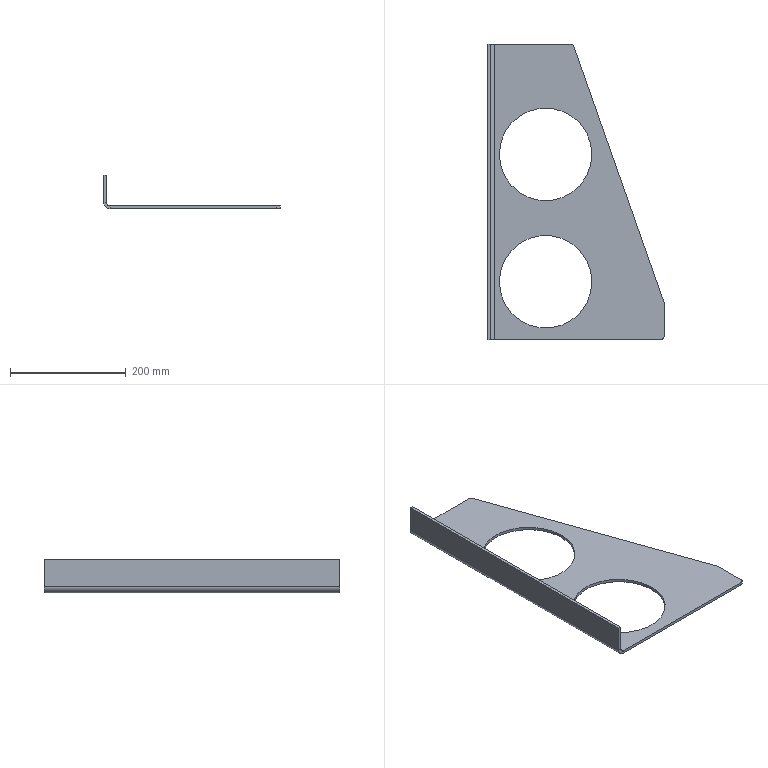Part | SolidWorks | features EdgeFlange 1, FlatPattern 1, ICE 1, SMBaseFlange 1, SheetMetal 1, UnFold 1 | 1 solid | 22 faces | box 305 x 510 x 58 mm | volume 526681 mm3 | plane 13 | cylinder 9 | commonest cylinder face diameters 160 x4 14 x3 12 x1 22 x1
STEP:
#1=CARTESIAN_POINT('',(415.,110.,-5.));
#2=VERTEX_POINT('',#1);
#3=CARTESIAN_POINT('',(255.,110.,-5.));
#4=VERTEX_POINT('',#3);
#5=CARTESIAN_POINT('',(335.,110.,-5.));
#6=DIRECTION('',(0.,0.,-1.));
#7=DIRECTION('',(-1.,0.,0.));
#8=AXIS2_PLACEMENT_3D('',#5,#6,#7);
#9=CIRCLE('',#8,80.);
#10=EDGE_CURVE('',#2,#4,#9,.T.);
#11=ORIENTED_EDGE('',*,*,#10,.T.);
#12=CARTESIAN_POINT('',(255.,110.,0.));
#13=VERTEX_POINT('',#12);
#14=CARTESIAN_POINT('',(255.,110.,-10.));
#15=DIRECTION('',(0.,0.,1.));
#16=VECTOR('',#15,1000.);
#17=LINE('',#14,#16);
#18=EDGE_CURVE('',#4,#13,#17,.T.);
#19=ORIENTED_EDGE('',*,*,#18,.T.);
#20=CARTESIAN_POINT('',(415.,110.,0.));
#21=VERTEX_POINT('',#20);
#22=CARTESIAN_POINT('',(335.,110.,0.));
#23=DIRECTION('',(0.,0.,1.));
#24=DIRECTION('',(1.,0.,0.));
#25=AXIS2_PLACEMENT_3D('',#22,#23,#24);
#26=CIRCLE('',#25,80.);
#27=EDGE_CURVE('',#13,#21,#26,.T.);
#28=ORIENTED_EDGE('',*,*,#27,.T.);
#29=CARTESIAN_POINT('',(415.,110.,-10.));
#30=DIRECTION('',(0.,0.,1.));
#31=VECTOR('',#30,1000.);
#32=LINE('',#29,#31);
#33=EDGE_CURVE('',#2,#21,#32,.T.);
#34=ORIENTED_EDGE('',*,*,#33,.F.);
#35=EDGE_LOOP('',(#11,#19,#28,#34));
#36=FACE_OUTER_BOUND('',#35,.T.);
#37=CARTESIAN_POINT('',(335.,110.,-10.));
#38=DIRECTION('',(0.,0.,1.));
#39=DIRECTION('',(1.,0.,0.));
#40=AXIS2_PLACEMENT_3D('',#37,#38,#39);
#41=CYLINDRICAL_SURFACE('',#40,80.);
#42=ADVANCED_FACE('',(#36),#41,.F.);
#43=CARTESIAN_POINT('',(415.,330.,-5.));
#44=VERTEX_POINT('',#43);
#45=CARTESIAN_POINT('',(255.,330.,-5.));
#46=VERTEX_POINT('',#45);
#47=CARTESIAN_POINT('',(335.,330.,-5.));
#48=DIRECTION('',(0.,0.,-1.));
#49=DIRECTION('',(-1.,0.,0.));
#50=AXIS2_PLACEMENT_3D('',#47,#48,#49);
#51=CIRCLE('',#50,80.);
#52=EDGE_CURVE('',#44,#46,#51,.T.);
#53=ORIENTED_EDGE('',*,*,#52,.T.);
#54=CARTESIAN_POINT('',(255.,330.,0.));
#55=VERTEX_POINT('',#54);
#56=CARTESIAN_POINT('',(255.,330.,-10.));
#57=DIRECTION('',(0.,0.,1.));
#58=VECTOR('',#57,1000.);
#59=LINE('',#56,#58);
#60=EDGE_CURVE('',#46,#55,#59,.T.);
#61=ORIENTED_EDGE('',*,*,#60,.T.);
#62=CARTESIAN_POINT('',(415.,330.,0.));
#63=VERTEX_POINT('',#62);
#64=CARTESIAN_POINT('',(335.,330.,0.));
#65=DIRECTION('',(0.,0.,1.));
#66=DIRECTION('',(1.,0.,0.));
#67=AXIS2_PLACEMENT_3D('',#64,#65,#66);
#68=CIRCLE('',#67,80.);
#69=EDGE_CURVE('',#55,#63,#68,.T.);
#70=ORIENTED_EDGE('',*,*,#69,.T.);
#71=CARTESIAN_POINT('',(415.,330.,-10.));
#72=DIRECTION('',(0.,0.,1.));
#73=VECTOR('',#72,1000.);
#74=LINE('',#71,#73);
#75=EDGE_CURVE('',#44,#63,#74,.T.);
#76=ORIENTED_EDGE('',*,*,#75,.F.);
#77=EDGE_LOOP('',(#53,#61,#70,#76));
#78=FACE_OUTER_BOUND('',#77,.T.);
#79=CARTESIAN_POINT('',(335.,330.,-10.));
#80=DIRECTION('',(0.,0.,1.));
#81=DIRECTION('',(1.,0.,0.));
#82=AXIS2_PLACEMENT_3D('',#79,#80,#81);
#83=CYLINDRICAL_SURFACE('',#82,80.);
#84=ADVANCED_FACE('',(#78),#83,.F.);
#85=CARTESIAN_POINT('',(246.,10.,0.));
#86=VERTEX_POINT('',#85);
#87=CARTESIAN_POINT('',(533.,10.,0.));
#88=VERTEX_POINT('',#87);
#89=CARTESIAN_POINT('',(235.,10.,0.));
#90=DIRECTION('',(1.,0.,0.));
#91=VECTOR('',#90,1000.);
#92=LINE('',#89,#91);
#93=EDGE_CURVE('',#86,#88,#92,.T.);
#94=ORIENTED_EDGE('',*,*,#93,.F.);
#95=CARTESIAN_POINT('',(246.,10.,-5.));
#96=VERTEX_POINT('',#95);
#97=CARTESIAN_POINT('',(246.,10.,0.));
#98=DIRECTION('',(0.,0.,-1.));
#99=VECTOR('',#98,1000.);
#100=LINE('',#97,#99);
#101=EDGE_CURVE('',#86,#96,#100,.T.);
#102=ORIENTED_EDGE('',*,*,#101,.T.);
#103=CARTESIAN_POINT('',(533.,10.,-5.));
#104=VERTEX_POINT('',#103);
#105=CARTESIAN_POINT('',(235.,10.,-5.));
#106=DIRECTION('',(1.,0.,0.));
#107=VECTOR('',#106,1000.);
#108=LINE('',#105,#107);
#109=EDGE_CURVE('',#96,#104,#108,.T.);
#110=ORIENTED_EDGE('',*,*,#109,.T.);
#111=CARTESIAN_POINT('',(533.,10.,-5.));
#112=DIRECTION('',(0.,0.,1.));
#113=VECTOR('',#112,1000.);
#114=LINE('',#111,#113);
#115=EDGE_CURVE('',#104,#88,#114,.T.);
#116=ORIENTED_EDGE('',*,*,#115,.T.);
#117=EDGE_LOOP('',(#94,#102,#110,#116));
#118=FACE_OUTER_BOUND('',#117,.T.);
#119=CARTESIAN_POINT('',(235.,10.,-5.));
#120=DIRECTION('',(0.,-1.,0.));
#121=DIRECTION('',(0.,0.,-1.));
#122=AXIS2_PLACEMENT_3D('',#119,#120,#121);
#123=PLANE('',#122);
#124=ADVANCED_FACE('',(#118),#123,.T.);
#125=ORIENTED_EDGE('',*,*,#10,.F.);
#126=CARTESIAN_POINT('',(335.,110.,-5.));
#127=DIRECTION('',(0.,0.,-1.));
#128=DIRECTION('',(-1.,0.,0.));
#129=AXIS2_PLACEMENT_3D('',#126,#127,#128);
#130=CIRCLE('',#129,80.);
#131=EDGE_CURVE('',#4,#2,#130,.T.);
#132=ORIENTED_EDGE('',*,*,#131,.F.);
#133=EDGE_LOOP('',(#125,#132));
#134=FACE_BOUND('',#133,.T.);
#135=ORIENTED_EDGE('',*,*,#52,.F.);
#136=CARTESIAN_POINT('',(335.,330.,-5.));
#137=DIRECTION('',(0.,0.,-1.));
#138=DIRECTION('',(-1.,0.,0.));
#139=AXIS2_PLACEMENT_3D('',#136,#137,#138);
#140=CIRCLE('',#139,80.);
#141=EDGE_CURVE('',#46,#44,#140,.T.);
#142=ORIENTED_EDGE('',*,*,#141,.F.);
#143=EDGE_LOOP('',(#135,#142));
#144=FACE_BOUND('',#143,.T.);
#145=ORIENTED_EDGE('',*,*,#109,.F.);
#146=CARTESIAN_POINT('',(246.,520.,-5.));
#147=VERTEX_POINT('',#146);
#148=CARTESIAN_POINT('',(246.,10.,-5.));
#149=DIRECTION('',(0.,1.,0.));
#150=VECTOR('',#149,1000.);
#151=LINE('',#148,#150);
#152=EDGE_CURVE('',#96,#147,#151,.T.);
#153=ORIENTED_EDGE('',*,*,#152,.T.);
#154=CARTESIAN_POINT('',(377.818,520.,-5.));
#155=VERTEX_POINT('',#154);
#156=CARTESIAN_POINT('',(235.,520.,-5.));
#157=DIRECTION('',(-1.,0.,0.));
#158=VECTOR('',#157,1000.);
#159=LINE('',#156,#158);
#160=EDGE_CURVE('',#155,#147,#159,.T.);
#161=ORIENTED_EDGE('',*,*,#160,.F.);
#162=CARTESIAN_POINT('',(384.422,515.322,-5.));
#163=VERTEX_POINT('',#162);
#164=CARTESIAN_POINT('',(377.818,513.,-5.));
#165=DIRECTION('',(0.,0.,1.));
#166=DIRECTION('',(1.,0.,0.));
#167=AXIS2_PLACEMENT_3D('',#164,#165,#166);
#168=CIRCLE('',#167,7.);
#169=EDGE_CURVE('',#163,#155,#168,.T.);
#170=ORIENTED_EDGE('',*,*,#169,.F.);
#171=CARTESIAN_POINT('',(539.604,73.92,-5.));
#172=VERTEX_POINT('',#171);
#173=CARTESIAN_POINT('',(384.422,515.322,-5.));
#174=DIRECTION('',(-0.3317,0.9434,0.));
#175=VECTOR('',#174,1000.);
#176=LINE('',#173,#175);
#177=EDGE_CURVE('',#172,#163,#176,.T.);
#178=ORIENTED_EDGE('',*,*,#177,.F.);
#179=CARTESIAN_POINT('',(540.,71.599,-5.));
#180=VERTEX_POINT('',#179);
#181=CARTESIAN_POINT('',(533.,71.599,-5.));
#182=DIRECTION('',(0.,0.,1.));
#183=DIRECTION('',(1.,0.,0.));
#184=AXIS2_PLACEMENT_3D('',#181,#182,#183);
#185=CIRCLE('',#184,7.);
#186=EDGE_CURVE('',#180,#172,#185,.T.);
#187=ORIENTED_EDGE('',*,*,#186,.F.);
#188=CARTESIAN_POINT('',(540.,17.,-5.));
#189=VERTEX_POINT('',#188);
#190=CARTESIAN_POINT('',(540.,17.,-5.));
#191=DIRECTION('',(0.,1.,0.));
#192=VECTOR('',#191,1000.);
#193=LINE('',#190,#192);
#194=EDGE_CURVE('',#189,#180,#193,.T.);
#195=ORIENTED_EDGE('',*,*,#194,.F.);
#196=CARTESIAN_POINT('',(533.,17.,-5.));
#197=DIRECTION('',(0.,0.,1.));
#198=DIRECTION('',(-1.,0.,0.));
#199=AXIS2_PLACEMENT_3D('',#196,#197,#198);
#200=CIRCLE('',#199,7.);
#201=EDGE_CURVE('',#104,#189,#200,.T.);
#202=ORIENTED_EDGE('',*,*,#201,.F.);
#203=EDGE_LOOP('',(#145,#153,#161,#170,#178,#187,#195,#202));
#204=FACE_OUTER_BOUND('',#203,.T.);
#205=CARTESIAN_POINT('',(533.,17.,-5.));
#206=DIRECTION('',(0.,0.,-1.));
#207=DIRECTION('',(-1.,0.,0.));
#208=AXIS2_PLACEMENT_3D('',#205,#206,#207);
#209=PLANE('',#208);
#210=ADVANCED_FACE('',(#134,#144,#204),#209,.T.);
#211=CARTESIAN_POINT('',(335.,330.,0.));
#212=DIRECTION('',(0.,0.,1.));
#213=DIRECTION('',(1.,0.,0.));
#214=AXIS2_PLACEMENT_3D('',#211,#212,#213);
#215=CIRCLE('',#214,80.);
#216=EDGE_CURVE('',#63,#55,#215,.T.);
#217=ORIENTED_EDGE('',*,*,#216,.F.);
#218=ORIENTED_EDGE('',*,*,#69,.F.);
#219=EDGE_LOOP('',(#217,#218));
#220=FACE_BOUND('',#219,.T.);
#221=CARTESIAN_POINT('',(335.,110.,0.));
#222=DIRECTION('',(0.,0.,1.));
#223=DIRECTION('',(1.,0.,0.));
#224=AXIS2_PLACEMENT_3D('',#221,#222,#223);
#225=CIRCLE('',#224,80.);
#226=EDGE_CURVE('',#21,#13,#225,.T.);
#227=ORIENTED_EDGE('',*,*,#226,.F.);
#228=ORIENTED_EDGE('',*,*,#27,.F.);
#229=EDGE_LOOP('',(#227,#228));
#230=FACE_BOUND('',#229,.T.);
#231=CARTESIAN_POINT('',(246.,520.,0.));
#232=VERTEX_POINT('',#231);
#233=CARTESIAN_POINT('',(246.,10.,0.));
#234=DIRECTION('',(0.,1.,0.));
#235=VECTOR('',#234,1000.);
#236=LINE('',#233,#235);
#237=EDGE_CURVE('',#86,#232,#236,.T.);
#238=ORIENTED_EDGE('',*,*,#237,.F.);
#239=ORIENTED_EDGE('',*,*,#93,.T.);
#240=CARTESIAN_POINT('',(540.,17.,0.));
#241=VERTEX_POINT('',#240);
#242=CARTESIAN_POINT('',(533.,17.,0.));
#243=DIRECTION('',(0.,0.,1.));
#244=DIRECTION('',(-1.,0.,0.));
#245=AXIS2_PLACEMENT_3D('',#242,#243,#244);
#246=CIRCLE('',#245,7.);
#247=EDGE_CURVE('',#88,#241,#246,.T.);
#248=ORIENTED_EDGE('',*,*,#247,.T.);
#249=CARTESIAN_POINT('',(540.,71.599,0.));
#250=VERTEX_POINT('',#249);
#251=CARTESIAN_POINT('',(540.,17.,0.));
#252=DIRECTION('',(0.,1.,0.));
#253=VECTOR('',#252,1000.);
#254=LINE('',#251,#253);
#255=EDGE_CURVE('',#241,#250,#254,.T.);
#256=ORIENTED_EDGE('',*,*,#255,.T.);
#257=CARTESIAN_POINT('',(539.604,73.92,0.));
#258=VERTEX_POINT('',#257);
#259=CARTESIAN_POINT('',(533.,71.599,0.));
#260=DIRECTION('',(0.,0.,1.));
#261=DIRECTION('',(1.,0.,0.));
#262=AXIS2_PLACEMENT_3D('',#259,#260,#261);
#263=CIRCLE('',#262,7.);
#264=EDGE_CURVE('',#250,#258,#263,.T.);
#265=ORIENTED_EDGE('',*,*,#264,.T.);
#266=CARTESIAN_POINT('',(384.422,515.322,0.));
#267=VERTEX_POINT('',#266);
#268=CARTESIAN_POINT('',(384.422,515.322,0.));
#269=DIRECTION('',(-0.3317,0.9434,0.));
#270=VECTOR('',#269,1000.);
#271=LINE('',#268,#270);
#272=EDGE_CURVE('',#258,#267,#271,.T.);
#273=ORIENTED_EDGE('',*,*,#272,.T.);
#274=CARTESIAN_POINT('',(377.818,520.,0.));
#275=VERTEX_POINT('',#274);
#276=CARTESIAN_POINT('',(377.818,513.,0.));
#277=DIRECTION('',(0.,0.,1.));
#278=DIRECTION('',(1.,0.,0.));
#279=AXIS2_PLACEMENT_3D('',#276,#277,#278);
#280=CIRCLE('',#279,7.);
#281=EDGE_CURVE('',#267,#275,#280,.T.);
#282=ORIENTED_EDGE('',*,*,#281,.T.);
#283=CARTESIAN_POINT('',(235.,520.,0.));
#284=DIRECTION('',(-1.,0.,0.));
#285=VECTOR('',#284,1000.);
#286=LINE('',#283,#285);
#287=EDGE_CURVE('',#275,#232,#286,.T.);
#288=ORIENTED_EDGE('',*,*,#287,.T.);
#289=EDGE_LOOP('',(#238,#239,#248,#256,#265,#273,#282,#288));
#290=FACE_OUTER_BOUND('',#289,.T.);
#291=CARTESIAN_POINT('',(533.,17.,0.));
#292=DIRECTION('',(0.,0.,-1.));
#293=DIRECTION('',(-1.,0.,0.));
#294=AXIS2_PLACEMENT_3D('',#291,#292,#293);
#295=PLANE('',#294);
#296=ADVANCED_FACE('',(#220,#230,#290),#295,.F.);
#297=CARTESIAN_POINT('',(246.,520.,0.));
#298=DIRECTION('',(0.,0.,-1.));
#299=VECTOR('',#298,1000.);
#300=LINE('',#297,#299);
#301=EDGE_CURVE('',#232,#147,#300,.T.);
#302=ORIENTED_EDGE('',*,*,#301,.F.);
#303=ORIENTED_EDGE('',*,*,#287,.F.);
#304=CARTESIAN_POINT('',(377.818,520.,-5.));
#305=DIRECTION('',(0.,0.,1.));
#306=VECTOR('',#305,1000.);
#307=LINE('',#304,#306);
#308=EDGE_CURVE('',#155,#275,#307,.T.);
#309=ORIENTED_EDGE('',*,*,#308,.F.);
#310=ORIENTED_EDGE('',*,*,#160,.T.);
#311=EDGE_LOOP('',(#302,#303,#309,#310));
#312=FACE_OUTER_BOUND('',#311,.T.);
#313=CARTESIAN_POINT('',(235.,520.,-5.));
#314=DIRECTION('',(0.,1.,0.));
#315=DIRECTION('',(-1.,0.,0.));
#316=AXIS2_PLACEMENT_3D('',#313,#314,#315);
#317=PLANE('',#316);
#318=ADVANCED_FACE('',(#312),#317,.T.);
#319=ORIENTED_EDGE('',*,*,#281,.F.);
#320=CARTESIAN_POINT('',(384.422,515.322,-5.));
#321=DIRECTION('',(0.,0.,1.));
#322=VECTOR('',#321,1000.);
#323=LINE('',#320,#322);
#324=EDGE_CURVE('',#163,#267,#323,.T.);
#325=ORIENTED_EDGE('',*,*,#324,.F.);
#326=ORIENTED_EDGE('',*,*,#169,.T.);
#327=ORIENTED_EDGE('',*,*,#308,.T.);
#328=EDGE_LOOP('',(#319,#325,#326,#327));
#329=FACE_OUTER_BOUND('',#328,.T.);
#330=CARTESIAN_POINT('',(377.818,513.,-5.));
#331=DIRECTION('',(0.,0.,1.));
#332=DIRECTION('',(1.,0.,0.));
#333=AXIS2_PLACEMENT_3D('',#330,#331,#332);
#334=CYLINDRICAL_SURFACE('',#333,7.);
#335=ADVANCED_FACE('',(#329),#334,.T.);
#336=ORIENTED_EDGE('',*,*,#272,.F.);
#337=CARTESIAN_POINT('',(539.604,73.92,-5.));
#338=DIRECTION('',(0.,0.,1.));
#339=VECTOR('',#338,1000.);
#340=LINE('',#337,#339);
#341=EDGE_CURVE('',#172,#258,#340,.T.);
#342=ORIENTED_EDGE('',*,*,#341,.F.);
#343=ORIENTED_EDGE('',*,*,#177,.T.);
#344=ORIENTED_EDGE('',*,*,#324,.T.);
#345=EDGE_LOOP('',(#336,#342,#343,#344));
#346=FACE_OUTER_BOUND('',#345,.T.);
#347=CARTESIAN_POINT('',(384.422,515.322,-5.));
#348=DIRECTION('',(0.9434,0.3317,0.));
#349=DIRECTION('',(-0.3317,0.9434,0.));
#350=AXIS2_PLACEMENT_3D('',#347,#348,#349);
#351=PLANE('',#350);
#352=ADVANCED_FACE('',(#346),#351,.T.);
#353=ORIENTED_EDGE('',*,*,#264,.F.);
#354=CARTESIAN_POINT('',(540.,71.599,-5.));
#355=DIRECTION('',(0.,0.,1.));
#356=VECTOR('',#355,1000.);
#357=LINE('',#354,#356);
#358=EDGE_CURVE('',#180,#250,#357,.T.);
#359=ORIENTED_EDGE('',*,*,#358,.F.);
#360=ORIENTED_EDGE('',*,*,#186,.T.);
#361=ORIENTED_EDGE('',*,*,#341,.T.);
#362=EDGE_LOOP('',(#353,#359,#360,#361));
#363=FACE_OUTER_BOUND('',#362,.T.);
#364=CARTESIAN_POINT('',(533.,71.599,-5.));
#365=DIRECTION('',(0.,0.,1.));
#366=DIRECTION('',(1.,0.,0.));
#367=AXIS2_PLACEMENT_3D('',#364,#365,#366);
#368=CYLINDRICAL_SURFACE('',#367,7.);
#369=ADVANCED_FACE('',(#363),#368,.T.);
#370=ORIENTED_EDGE('',*,*,#255,.F.);
#371=CARTESIAN_POINT('',(540.,17.,-5.));
#372=DIRECTION('',(0.,0.,1.));
#373=VECTOR('',#372,1000.);
#374=LINE('',#371,#373);
#375=EDGE_CURVE('',#189,#241,#374,.T.);
#376=ORIENTED_EDGE('',*,*,#375,.F.);
#377=ORIENTED_EDGE('',*,*,#194,.T.);
#378=ORIENTED_EDGE('',*,*,#358,.T.);
#379=EDGE_LOOP('',(#370,#376,#377,#378));
#380=FACE_OUTER_BOUND('',#379,.T.);
#381=CARTESIAN_POINT('',(540.,17.,-5.));
#382=DIRECTION('',(1.,0.,0.));
#383=DIRECTION('',(0.,1.,0.));
#384=AXIS2_PLACEMENT_3D('',#381,#382,#383);
#385=PLANE('',#384);
#386=ADVANCED_FACE('',(#380),#385,.T.);
#387=ORIENTED_EDGE('',*,*,#247,.F.);
#388=ORIENTED_EDGE('',*,*,#115,.F.);
#389=ORIENTED_EDGE('',*,*,#201,.T.);
#390=ORIENTED_EDGE('',*,*,#375,.T.);
#391=EDGE_LOOP('',(#387,#388,#389,#390));
#392=FACE_OUTER_BOUND('',#391,.T.);
#393=CARTESIAN_POINT('',(533.,17.,-5.));
#394=DIRECTION('',(0.,0.,1.));
#395=DIRECTION('',(1.,0.,0.));
#396=AXIS2_PLACEMENT_3D('',#393,#394,#395);
#397=CYLINDRICAL_SURFACE('',#396,7.);
#398=ADVANCED_FACE('',(#392),#397,.T.);
#399=ORIENTED_EDGE('',*,*,#60,.F.);
#400=ORIENTED_EDGE('',*,*,#141,.T.);
#401=ORIENTED_EDGE('',*,*,#75,.T.);
#402=ORIENTED_EDGE('',*,*,#216,.T.);
#403=EDGE_LOOP('',(#399,#400,#401,#402));
#404=FACE_OUTER_BOUND('',#403,.T.);
#405=CARTESIAN_POINT('',(335.,330.,-10.));
#406=DIRECTION('',(0.,0.,1.));
#407=DIRECTION('',(1.,0.,0.));
#408=AXIS2_PLACEMENT_3D('',#405,#406,#407);
#409=CYLINDRICAL_SURFACE('',#408,80.);
#410=ADVANCED_FACE('',(#404),#409,.F.);
#411=ORIENTED_EDGE('',*,*,#18,.F.);
#412=ORIENTED_EDGE('',*,*,#131,.T.);
#413=ORIENTED_EDGE('',*,*,#33,.T.);
#414=ORIENTED_EDGE('',*,*,#226,.T.);
#415=EDGE_LOOP('',(#411,#412,#413,#414));
#416=FACE_OUTER_BOUND('',#415,.T.);
#417=CARTESIAN_POINT('',(335.,110.,-10.));
#418=DIRECTION('',(0.,0.,1.));
#419=DIRECTION('',(1.,0.,0.));
#420=AXIS2_PLACEMENT_3D('',#417,#418,#419);
#421=CYLINDRICAL_SURFACE('',#420,80.);
#422=ADVANCED_FACE('',(#416),#421,.F.);
#423=CARTESIAN_POINT('',(240.,520.,6.));
#424=VERTEX_POINT('',#423);
#425=CARTESIAN_POINT('',(235.,520.,6.));
#426=VERTEX_POINT('',#425);
#427=CARTESIAN_POINT('',(235.,520.,6.));
#428=DIRECTION('',(-1.,0.,0.));
#429=VECTOR('',#428,1000.);
#430=LINE('',#427,#429);
#431=EDGE_CURVE('',#424,#426,#430,.T.);
#432=ORIENTED_EDGE('',*,*,#431,.F.);
#433=CARTESIAN_POINT('',(246.,520.,6.));
#434=DIRECTION('',(0.,1.,0.));
#435=DIRECTION('',(0.,0.,-1.));
#436=AXIS2_PLACEMENT_3D('',#433,#434,#435);
#437=CIRCLE('',#436,6.);
#438=EDGE_CURVE('',#232,#424,#437,.T.);
#439=ORIENTED_EDGE('',*,*,#438,.F.);
#440=ORIENTED_EDGE('',*,*,#301,.T.);
#441=CARTESIAN_POINT('',(246.,520.,6.));
#442=DIRECTION('',(0.,1.,0.));
#443=DIRECTION('',(0.,0.,-1.));
#444=AXIS2_PLACEMENT_3D('',#441,#442,#443);
#445=CIRCLE('',#444,11.);
#446=EDGE_CURVE('',#147,#426,#445,.T.);
#447=ORIENTED_EDGE('',*,*,#446,.T.);
#448=EDGE_LOOP('',(#432,#439,#440,#447));
#449=FACE_OUTER_BOUND('',#448,.T.);
#450=CARTESIAN_POINT('',(246.,520.,6.));
#451=DIRECTION('',(0.,1.,0.));
#452=DIRECTION('',(0.,0.,1.));
#453=AXIS2_PLACEMENT_3D('',#450,#451,#452);
#454=PLANE('',#453);
#455=ADVANCED_FACE('',(#449),#454,.T.);
#456=CARTESIAN_POINT('',(240.,10.,6.));
#457=VERTEX_POINT('',#456);
#458=CARTESIAN_POINT('',(246.,10.,6.));
#459=DIRECTION('',(0.,-1.,0.));
#460=DIRECTION('',(0.,0.,-1.));
#461=AXIS2_PLACEMENT_3D('',#458,#459,#460);
#462=CIRCLE('',#461,6.);
#463=EDGE_CURVE('',#457,#86,#462,.T.);
#464=ORIENTED_EDGE('',*,*,#463,.F.);
#465=CARTESIAN_POINT('',(235.,10.,6.));
#466=VERTEX_POINT('',#465);
#467=CARTESIAN_POINT('',(240.,10.,6.));
#468=DIRECTION('',(-1.,0.,0.));
#469=VECTOR('',#468,1000.);
#470=LINE('',#467,#469);
#471=EDGE_CURVE('',#457,#466,#470,.T.);
#472=ORIENTED_EDGE('',*,*,#471,.T.);
#473=CARTESIAN_POINT('',(246.,10.,6.));
#474=DIRECTION('',(0.,-1.,0.));
#475=DIRECTION('',(0.,0.,-1.));
#476=AXIS2_PLACEMENT_3D('',#473,#474,#475);
#477=CIRCLE('',#476,11.);
#478=EDGE_CURVE('',#466,#96,#477,.T.);
#479=ORIENTED_EDGE('',*,*,#478,.T.);
#480=ORIENTED_EDGE('',*,*,#101,.F.);
#481=EDGE_LOOP('',(#464,#472,#479,#480));
#482=FACE_OUTER_BOUND('',#481,.T.);
#483=CARTESIAN_POINT('',(246.,10.,6.));
#484=DIRECTION('',(0.,1.,0.));
#485=DIRECTION('',(0.,0.,1.));
#486=AXIS2_PLACEMENT_3D('',#483,#484,#485);
#487=PLANE('',#486);
#488=ADVANCED_FACE('',(#482),#487,.F.);
#489=ORIENTED_EDGE('',*,*,#152,.F.);
#490=ORIENTED_EDGE('',*,*,#478,.F.);
#491=CARTESIAN_POINT('',(235.,0.,6.));
#492=DIRECTION('',(0.,-1.,0.));
#493=VECTOR('',#492,1000.);
#494=LINE('',#491,#493);
#495=EDGE_CURVE('',#426,#466,#494,.T.);
#496=ORIENTED_EDGE('',*,*,#495,.F.);
#497=ORIENTED_EDGE('',*,*,#446,.F.);
#498=EDGE_LOOP('',(#489,#490,#496,#497));
#499=FACE_OUTER_BOUND('',#498,.T.);
#500=CARTESIAN_POINT('',(246.,10.,6.));
#501=DIRECTION('',(0.,-1.,0.));
#502=DIRECTION('',(-1.,0.,0.));
#503=AXIS2_PLACEMENT_3D('',#500,#501,#502);
#504=CYLINDRICAL_SURFACE('',#503,11.);
#505=ADVANCED_FACE('',(#499),#504,.T.);
#506=ORIENTED_EDGE('',*,*,#237,.T.);
#507=ORIENTED_EDGE('',*,*,#438,.T.);
#508=CARTESIAN_POINT('',(240.,520.,6.));
#509=DIRECTION('',(0.,-1.,0.));
#510=VECTOR('',#509,1000.);
#511=LINE('',#508,#510);
#512=EDGE_CURVE('',#424,#457,#511,.T.);
#513=ORIENTED_EDGE('',*,*,#512,.T.);
#514=ORIENTED_EDGE('',*,*,#463,.T.);
#515=EDGE_LOOP('',(#506,#507,#513,#514));
#516=FACE_OUTER_BOUND('',#515,.T.);
#517=CARTESIAN_POINT('',(246.,10.,6.));
#518=DIRECTION('',(0.,-1.,0.));
#519=DIRECTION('',(-1.,0.,0.));
#520=AXIS2_PLACEMENT_3D('',#517,#518,#519);
#521=CYLINDRICAL_SURFACE('',#520,6.);
#522=ADVANCED_FACE('',(#516),#521,.F.);
#523=CARTESIAN_POINT('',(235.,10.,53.));
#524=VERTEX_POINT('',#523);
#525=CARTESIAN_POINT('',(235.,10.,0.));
#526=DIRECTION('',(0.,0.,-1.));
#527=VECTOR('',#526,1000.);
#528=LINE('',#525,#527);
#529=EDGE_CURVE('',#524,#466,#528,.T.);
#530=ORIENTED_EDGE('',*,*,#529,.T.);
#531=ORIENTED_EDGE('',*,*,#471,.F.);
#532=CARTESIAN_POINT('',(240.,10.,53.));
#533=VERTEX_POINT('',#532);
#534=CARTESIAN_POINT('',(240.,10.,0.));
#535=DIRECTION('',(0.,0.,-1.));
#536=VECTOR('',#535,1000.);
#537=LINE('',#534,#536);
#538=EDGE_CURVE('',#533,#457,#537,.T.);
#539=ORIENTED_EDGE('',*,*,#538,.F.);
#540=CARTESIAN_POINT('',(235.,10.,53.));
#541=DIRECTION('',(1.,0.,0.));
#542=VECTOR('',#541,1000.);
#543=LINE('',#540,#542);
#544=EDGE_CURVE('',#524,#533,#543,.T.);
#545=ORIENTED_EDGE('',*,*,#544,.F.);
#546=EDGE_LOOP('',(#530,#531,#539,#545));
#547=FACE_OUTER_BOUND('',#546,.T.);
#548=CARTESIAN_POINT('',(235.,10.,0.));
#549=DIRECTION('',(0.,-1.,0.));
#550=DIRECTION('',(0.,0.,-1.));
#551=AXIS2_PLACEMENT_3D('',#548,#549,#550);
#552=PLANE('',#551);
#553=ADVANCED_FACE('',(#547),#552,.T.);
#554=CARTESIAN_POINT('',(240.,520.,53.));
#555=VERTEX_POINT('',#554);
#556=CARTESIAN_POINT('',(240.,520.,0.));
#557=DIRECTION('',(0.,0.,1.));
#558=VECTOR('',#557,1000.);
#559=LINE('',#556,#558);
#560=EDGE_CURVE('',#424,#555,#559,.T.);
#561=ORIENTED_EDGE('',*,*,#560,.F.);
#562=ORIENTED_EDGE('',*,*,#431,.T.);
#563=CARTESIAN_POINT('',(235.,520.,53.));
#564=VERTEX_POINT('',#563);
#565=CARTESIAN_POINT('',(235.,520.,53.));
#566=DIRECTION('',(0.,0.,1.));
#567=VECTOR('',#566,1000.);
#568=LINE('',#565,#567);
#569=EDGE_CURVE('',#426,#564,#568,.T.);
#570=ORIENTED_EDGE('',*,*,#569,.T.);
#571=CARTESIAN_POINT('',(235.,520.,53.));
#572=DIRECTION('',(1.,0.,0.));
#573=VECTOR('',#572,1000.);
#574=LINE('',#571,#573);
#575=EDGE_CURVE('',#564,#555,#574,.T.);
#576=ORIENTED_EDGE('',*,*,#575,.T.);
#577=EDGE_LOOP('',(#561,#562,#570,#576));
#578=FACE_OUTER_BOUND('',#577,.T.);
#579=CARTESIAN_POINT('',(235.,520.,53.));
#580=DIRECTION('',(0.,1.,0.));
#581=DIRECTION('',(-1.,0.,0.));
#582=AXIS2_PLACEMENT_3D('',#579,#580,#581);
#583=PLANE('',#582);
#584=ADVANCED_FACE('',(#578),#583,.T.);
#585=ORIENTED_EDGE('',*,*,#569,.F.);
#586=ORIENTED_EDGE('',*,*,#495,.T.);
#587=ORIENTED_EDGE('',*,*,#529,.F.);
#588=CARTESIAN_POINT('',(235.,10.,53.));
#589=DIRECTION('',(0.,-1.,0.));
#590=VECTOR('',#589,1000.);
#591=LINE('',#588,#590);
#592=EDGE_CURVE('',#564,#524,#591,.T.);
#593=ORIENTED_EDGE('',*,*,#592,.F.);
#594=EDGE_LOOP('',(#585,#586,#587,#593));
#595=FACE_OUTER_BOUND('',#594,.T.);
#596=CARTESIAN_POINT('',(235.,0.,0.));
#597=DIRECTION('',(-1.,0.,0.));
#598=DIRECTION('',(0.,0.,1.));
#599=AXIS2_PLACEMENT_3D('',#596,#597,#598);
#600=PLANE('',#599);
#601=ADVANCED_FACE('',(#595),#600,.T.);
#602=ORIENTED_EDGE('',*,*,#512,.F.);
#603=ORIENTED_EDGE('',*,*,#560,.T.);
#604=CARTESIAN_POINT('',(240.,0.,53.));
#605=DIRECTION('',(0.,-1.,0.));
#606=VECTOR('',#605,1000.);
#607=LINE('',#604,#606);
#608=EDGE_CURVE('',#555,#533,#607,.T.);
#609=ORIENTED_EDGE('',*,*,#608,.T.);
#610=ORIENTED_EDGE('',*,*,#538,.T.);
#611=EDGE_LOOP('',(#602,#603,#609,#610));
#612=FACE_OUTER_BOUND('',#611,.T.);
#613=CARTESIAN_POINT('',(240.,0.,0.));
#614=DIRECTION('',(-1.,0.,0.));
#615=DIRECTION('',(0.,0.,1.));
#616=AXIS2_PLACEMENT_3D('',#613,#614,#615);
#617=PLANE('',#616);
#618=ADVANCED_FACE('',(#612),#617,.F.);
#619=ORIENTED_EDGE('',*,*,#608,.F.);
#620=ORIENTED_EDGE('',*,*,#575,.F.);
#621=ORIENTED_EDGE('',*,*,#592,.T.);
#622=ORIENTED_EDGE('',*,*,#544,.T.);
#623=EDGE_LOOP('',(#619,#620,#621,#622));
#624=FACE_OUTER_BOUND('',#623,.T.);
#625=CARTESIAN_POINT('',(235.,10.,53.));
#626=DIRECTION('',(0.,0.,1.));
#627=DIRECTION('',(1.,0.,0.));
#628=AXIS2_PLACEMENT_3D('',#625,#626,#627);
#629=PLANE('',#628);
#630=ADVANCED_FACE('',(#624),#629,.T.);
#631=CLOSED_SHELL('',(#42,#84,#124,#210,#296,#318,#335,#352,#369,#386,#398,#410,#422,#455,#488,#505,#522,#553,#584,#601,#618,#630));
#632=MANIFOLD_SOLID_BREP('',#631);
#633=CARTESIAN_POINT('',(0.,0.,0.));
#634=DIRECTION('',(0.,0.,1.));
#635=DIRECTION('',(1.,0.,0.));
#636=AXIS2_PLACEMENT_3D('',#633,#634,#635);
#637=(LENGTH_UNIT()NAMED_UNIT(*)SI_UNIT(.MILLI.,.METRE.));
#638=UNCERTAINTY_MEASURE_WITH_UNIT(LENGTH_MEASURE(0.00001),#637,'','');
#639=(NAMED_UNIT(*)PLANE_ANGLE_UNIT()SI_UNIT($,.RADIAN.));
#640=(NAMED_UNIT(*)SI_UNIT($,.STERADIAN.)SOLID_ANGLE_UNIT());
#641=(GEOMETRIC_REPRESENTATION_CONTEXT(3)GLOBAL_UNCERTAINTY_ASSIGNED_CONTEXT((#638))GLOBAL_UNIT_ASSIGNED_CONTEXT((#637,#639,#640))REPRESENTATION_CONTEXT('',''));
#642=ADVANCED_BREP_SHAPE_REPRESENTATION('',(#632,#636),#641);